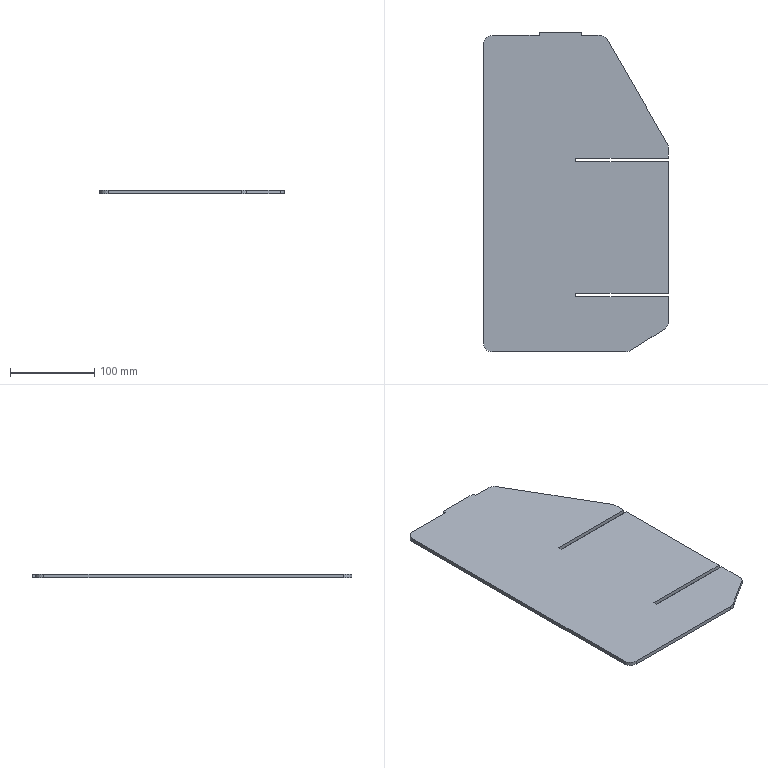Part | SolidWorks | features FlatPattern 1, SMBaseFlange 1, SheetMetal 1 | 1 solid | 26 faces | box 218.7 x 379.2 x 4.5 mm | volume 340357 mm3 | plane 20 | cylinder 6 | commonest cylinder face diameters 20 x6
STEP:
#1=CARTESIAN_POINT('',(18.5,-249.8,0.));
#2=VERTEX_POINT('',#1);
#3=CARTESIAN_POINT('',(8.5,-259.8,0.));
#4=VERTEX_POINT('',#3);
#5=CARTESIAN_POINT('',(18.5,-259.8,0.));
#6=DIRECTION('',(0.,0.,1.));
#7=DIRECTION('',(1.,0.,0.));
#8=AXIS2_PLACEMENT_3D('',#5,#6,#7);
#9=CIRCLE('',#8,10.);
#10=EDGE_CURVE('',#2,#4,#9,.T.);
#11=ORIENTED_EDGE('',*,*,#10,.F.);
#12=CARTESIAN_POINT('',(18.5,-249.8,-4.5));
#13=VERTEX_POINT('',#12);
#14=CARTESIAN_POINT('',(18.5,-249.8,-4.5));
#15=DIRECTION('',(0.,0.,1.));
#16=VECTOR('',#15,1000.);
#17=LINE('',#14,#16);
#18=EDGE_CURVE('',#13,#2,#17,.T.);
#19=ORIENTED_EDGE('',*,*,#18,.F.);
#20=CARTESIAN_POINT('',(8.5,-259.8,-4.5));
#21=VERTEX_POINT('',#20);
#22=CARTESIAN_POINT('',(18.5,-259.8,-4.5));
#23=DIRECTION('',(0.,0.,1.));
#24=DIRECTION('',(1.,0.,0.));
#25=AXIS2_PLACEMENT_3D('',#22,#23,#24);
#26=CIRCLE('',#25,10.);
#27=EDGE_CURVE('',#13,#21,#26,.T.);
#28=ORIENTED_EDGE('',*,*,#27,.T.);
#29=CARTESIAN_POINT('',(8.5,-259.8,-4.5));
#30=DIRECTION('',(0.,0.,1.));
#31=VECTOR('',#30,1000.);
#32=LINE('',#29,#31);
#33=EDGE_CURVE('',#21,#4,#32,.T.);
#34=ORIENTED_EDGE('',*,*,#33,.T.);
#35=EDGE_LOOP('',(#11,#19,#28,#34));
#36=FACE_OUTER_BOUND('',#35,.T.);
#37=CARTESIAN_POINT('',(18.5,-259.8,-4.5));
#38=DIRECTION('',(0.,0.,1.));
#39=DIRECTION('',(1.,0.,0.));
#40=AXIS2_PLACEMENT_3D('',#37,#38,#39);
#41=CYLINDRICAL_SURFACE('',#40,10.);
#42=ADVANCED_FACE('',(#36),#41,.T.);
#43=CARTESIAN_POINT('',(74.2,-249.8,0.));
#44=VERTEX_POINT('',#43);
#45=CARTESIAN_POINT('',(18.5,-249.8,0.));
#46=DIRECTION('',(-1.,0.,0.));
#47=VECTOR('',#46,1000.);
#48=LINE('',#45,#47);
#49=EDGE_CURVE('',#44,#2,#48,.T.);
#50=ORIENTED_EDGE('',*,*,#49,.F.);
#51=CARTESIAN_POINT('',(74.2,-249.8,-4.5));
#52=VERTEX_POINT('',#51);
#53=CARTESIAN_POINT('',(74.2,-249.8,-4.5));
#54=DIRECTION('',(0.,0.,1.));
#55=VECTOR('',#54,1000.);
#56=LINE('',#53,#55);
#57=EDGE_CURVE('',#52,#44,#56,.T.);
#58=ORIENTED_EDGE('',*,*,#57,.F.);
#59=CARTESIAN_POINT('',(18.5,-249.8,-4.5));
#60=DIRECTION('',(-1.,0.,0.));
#61=VECTOR('',#60,1000.);
#62=LINE('',#59,#61);
#63=EDGE_CURVE('',#52,#13,#62,.T.);
#64=ORIENTED_EDGE('',*,*,#63,.T.);
#65=ORIENTED_EDGE('',*,*,#18,.T.);
#66=EDGE_LOOP('',(#50,#58,#64,#65));
#67=FACE_OUTER_BOUND('',#66,.T.);
#68=CARTESIAN_POINT('',(18.5,-249.8,-4.5));
#69=DIRECTION('',(0.,1.,0.));
#70=DIRECTION('',(-1.,0.,0.));
#71=AXIS2_PLACEMENT_3D('',#68,#69,#70);
#72=PLANE('',#71);
#73=ADVANCED_FACE('',(#67),#72,.T.);
#74=CARTESIAN_POINT('',(74.2,-245.8,0.));
#75=VERTEX_POINT('',#74);
#76=CARTESIAN_POINT('',(74.2,-245.8,0.));
#77=DIRECTION('',(0.,-1.,0.));
#78=VECTOR('',#77,1000.);
#79=LINE('',#76,#78);
#80=EDGE_CURVE('',#75,#44,#79,.T.);
#81=ORIENTED_EDGE('',*,*,#80,.F.);
#82=CARTESIAN_POINT('',(74.2,-245.8,-4.5));
#83=VERTEX_POINT('',#82);
#84=CARTESIAN_POINT('',(74.2,-245.8,-4.5));
#85=DIRECTION('',(0.,0.,1.));
#86=VECTOR('',#85,1000.);
#87=LINE('',#84,#86);
#88=EDGE_CURVE('',#83,#75,#87,.T.);
#89=ORIENTED_EDGE('',*,*,#88,.F.);
#90=CARTESIAN_POINT('',(74.2,-245.8,-4.5));
#91=DIRECTION('',(0.,-1.,0.));
#92=VECTOR('',#91,1000.);
#93=LINE('',#90,#92);
#94=EDGE_CURVE('',#83,#52,#93,.T.);
#95=ORIENTED_EDGE('',*,*,#94,.T.);
#96=ORIENTED_EDGE('',*,*,#57,.T.);
#97=EDGE_LOOP('',(#81,#89,#95,#96));
#98=FACE_OUTER_BOUND('',#97,.T.);
#99=CARTESIAN_POINT('',(74.2,-245.8,-4.5));
#100=DIRECTION('',(-1.,0.,0.));
#101=DIRECTION('',(0.,0.,1.));
#102=AXIS2_PLACEMENT_3D('',#99,#100,#101);
#103=PLANE('',#102);
#104=ADVANCED_FACE('',(#98),#103,.T.);
#105=CARTESIAN_POINT('',(124.2,-245.8,0.));
#106=VERTEX_POINT('',#105);
#107=CARTESIAN_POINT('',(124.2,-245.8,0.));
#108=DIRECTION('',(-1.,0.,0.));
#109=VECTOR('',#108,1000.);
#110=LINE('',#107,#109);
#111=EDGE_CURVE('',#106,#75,#110,.T.);
#112=ORIENTED_EDGE('',*,*,#111,.F.);
#113=CARTESIAN_POINT('',(124.2,-245.8,-4.5));
#114=VERTEX_POINT('',#113);
#115=CARTESIAN_POINT('',(124.2,-245.8,-4.5));
#116=DIRECTION('',(0.,0.,1.));
#117=VECTOR('',#116,1000.);
#118=LINE('',#115,#117);
#119=EDGE_CURVE('',#114,#106,#118,.T.);
#120=ORIENTED_EDGE('',*,*,#119,.F.);
#121=CARTESIAN_POINT('',(124.2,-245.8,-4.5));
#122=DIRECTION('',(-1.,0.,0.));
#123=VECTOR('',#122,1000.);
#124=LINE('',#121,#123);
#125=EDGE_CURVE('',#114,#83,#124,.T.);
#126=ORIENTED_EDGE('',*,*,#125,.T.);
#127=ORIENTED_EDGE('',*,*,#88,.T.);
#128=EDGE_LOOP('',(#112,#120,#126,#127));
#129=FACE_OUTER_BOUND('',#128,.T.);
#130=CARTESIAN_POINT('',(124.2,-245.8,-4.5));
#131=DIRECTION('',(0.,1.,0.));
#132=DIRECTION('',(-1.,0.,0.));
#133=AXIS2_PLACEMENT_3D('',#130,#131,#132);
#134=PLANE('',#133);
#135=ADVANCED_FACE('',(#129),#134,.T.);
#136=CARTESIAN_POINT('',(124.2,-249.8,0.));
#137=VERTEX_POINT('',#136);
#138=CARTESIAN_POINT('',(124.2,-249.8,0.));
#139=DIRECTION('',(0.,1.,0.));
#140=VECTOR('',#139,1000.);
#141=LINE('',#138,#140);
#142=EDGE_CURVE('',#137,#106,#141,.T.);
#143=ORIENTED_EDGE('',*,*,#142,.F.);
#144=CARTESIAN_POINT('',(124.2,-249.8,-4.5));
#145=VERTEX_POINT('',#144);
#146=CARTESIAN_POINT('',(124.2,-249.8,-4.5));
#147=DIRECTION('',(0.,0.,1.));
#148=VECTOR('',#147,1000.);
#149=LINE('',#146,#148);
#150=EDGE_CURVE('',#145,#137,#149,.T.);
#151=ORIENTED_EDGE('',*,*,#150,.F.);
#152=CARTESIAN_POINT('',(124.2,-249.8,-4.5));
#153=DIRECTION('',(0.,1.,0.));
#154=VECTOR('',#153,1000.);
#155=LINE('',#152,#154);
#156=EDGE_CURVE('',#145,#114,#155,.T.);
#157=ORIENTED_EDGE('',*,*,#156,.T.);
#158=ORIENTED_EDGE('',*,*,#119,.T.);
#159=EDGE_LOOP('',(#143,#151,#157,#158));
#160=FACE_OUTER_BOUND('',#159,.T.);
#161=CARTESIAN_POINT('',(124.2,-249.8,-4.5));
#162=DIRECTION('',(1.,0.,0.));
#163=DIRECTION('',(0.,0.,-1.));
#164=AXIS2_PLACEMENT_3D('',#161,#162,#163);
#165=PLANE('',#164);
#166=ADVANCED_FACE('',(#160),#165,.T.);
#167=CARTESIAN_POINT('',(146.371,-249.8,0.));
#168=VERTEX_POINT('',#167);
#169=CARTESIAN_POINT('',(124.2,-249.8,0.));
#170=DIRECTION('',(-1.,0.,0.));
#171=VECTOR('',#170,1000.);
#172=LINE('',#169,#171);
#173=EDGE_CURVE('',#168,#137,#172,.T.);
#174=ORIENTED_EDGE('',*,*,#173,.F.);
#175=CARTESIAN_POINT('',(146.371,-249.8,-4.5));
#176=VERTEX_POINT('',#175);
#177=CARTESIAN_POINT('',(146.371,-249.8,-4.5));
#178=DIRECTION('',(0.,0.,1.));
#179=VECTOR('',#178,1000.);
#180=LINE('',#177,#179);
#181=EDGE_CURVE('',#176,#168,#180,.T.);
#182=ORIENTED_EDGE('',*,*,#181,.F.);
#183=CARTESIAN_POINT('',(124.2,-249.8,-4.5));
#184=DIRECTION('',(-1.,0.,0.));
#185=VECTOR('',#184,1000.);
#186=LINE('',#183,#185);
#187=EDGE_CURVE('',#176,#145,#186,.T.);
#188=ORIENTED_EDGE('',*,*,#187,.T.);
#189=ORIENTED_EDGE('',*,*,#150,.T.);
#190=EDGE_LOOP('',(#174,#182,#188,#189));
#191=FACE_OUTER_BOUND('',#190,.T.);
#192=CARTESIAN_POINT('',(124.2,-249.8,-4.5));
#193=DIRECTION('',(0.,1.,0.));
#194=DIRECTION('',(0.,0.,1.));
#195=AXIS2_PLACEMENT_3D('',#192,#193,#194);
#196=PLANE('',#195);
#197=ADVANCED_FACE('',(#191),#196,.T.);
#198=CARTESIAN_POINT('',(155.031,-254.8,0.));
#199=VERTEX_POINT('',#198);
#200=CARTESIAN_POINT('',(146.371,-259.8,0.));
#201=DIRECTION('',(0.,0.,1.));
#202=DIRECTION('',(-1.,0.,0.));
#203=AXIS2_PLACEMENT_3D('',#200,#201,#202);
#204=CIRCLE('',#203,10.);
#205=EDGE_CURVE('',#199,#168,#204,.T.);
#206=ORIENTED_EDGE('',*,*,#205,.F.);
#207=CARTESIAN_POINT('',(155.031,-254.8,-4.5));
#208=VERTEX_POINT('',#207);
#209=CARTESIAN_POINT('',(155.031,-254.8,-4.5));
#210=DIRECTION('',(0.,0.,1.));
#211=VECTOR('',#210,1000.);
#212=LINE('',#209,#211);
#213=EDGE_CURVE('',#208,#199,#212,.T.);
#214=ORIENTED_EDGE('',*,*,#213,.F.);
#215=CARTESIAN_POINT('',(146.371,-259.8,-4.5));
#216=DIRECTION('',(0.,0.,1.));
#217=DIRECTION('',(-1.,0.,0.));
#218=AXIS2_PLACEMENT_3D('',#215,#216,#217);
#219=CIRCLE('',#218,10.);
#220=EDGE_CURVE('',#208,#176,#219,.T.);
#221=ORIENTED_EDGE('',*,*,#220,.T.);
#222=ORIENTED_EDGE('',*,*,#181,.T.);
#223=EDGE_LOOP('',(#206,#214,#221,#222));
#224=FACE_OUTER_BOUND('',#223,.T.);
#225=CARTESIAN_POINT('',(146.371,-259.8,-4.5));
#226=DIRECTION('',(0.,0.,1.));
#227=DIRECTION('',(1.,0.,0.));
#228=AXIS2_PLACEMENT_3D('',#225,#226,#227);
#229=CYLINDRICAL_SURFACE('',#228,10.);
#230=ADVANCED_FACE('',(#224),#229,.T.);
#231=CARTESIAN_POINT('',(225.86,-377.479,0.));
#232=VERTEX_POINT('',#231);
#233=CARTESIAN_POINT('',(155.031,-254.8,0.));
#234=DIRECTION('',(-0.5,0.866,0.));
#235=VECTOR('',#234,1000.);
#236=LINE('',#233,#235);
#237=EDGE_CURVE('',#232,#199,#236,.T.);
#238=ORIENTED_EDGE('',*,*,#237,.F.);
#239=CARTESIAN_POINT('',(225.86,-377.479,-4.5));
#240=VERTEX_POINT('',#239);
#241=CARTESIAN_POINT('',(225.86,-377.479,-4.5));
#242=DIRECTION('',(0.,0.,1.));
#243=VECTOR('',#242,1000.);
#244=LINE('',#241,#243);
#245=EDGE_CURVE('',#240,#232,#244,.T.);
#246=ORIENTED_EDGE('',*,*,#245,.F.);
#247=CARTESIAN_POINT('',(155.031,-254.8,-4.5));
#248=DIRECTION('',(-0.5,0.866,0.));
#249=VECTOR('',#248,1000.);
#250=LINE('',#247,#249);
#251=EDGE_CURVE('',#240,#208,#250,.T.);
#252=ORIENTED_EDGE('',*,*,#251,.T.);
#253=ORIENTED_EDGE('',*,*,#213,.T.);
#254=EDGE_LOOP('',(#238,#246,#252,#253));
#255=FACE_OUTER_BOUND('',#254,.T.);
#256=CARTESIAN_POINT('',(155.031,-254.8,-4.5));
#257=DIRECTION('',(0.866,0.5,0.));
#258=DIRECTION('',(-0.5,0.866,0.));
#259=AXIS2_PLACEMENT_3D('',#256,#257,#258);
#260=PLANE('',#259);
#261=ADVANCED_FACE('',(#255),#260,.T.);
#262=CARTESIAN_POINT('',(227.2,-382.479,0.));
#263=VERTEX_POINT('',#262);
#264=CARTESIAN_POINT('',(217.2,-382.479,0.));
#265=DIRECTION('',(0.,0.,1.));
#266=DIRECTION('',(1.,0.,0.));
#267=AXIS2_PLACEMENT_3D('',#264,#265,#266);
#268=CIRCLE('',#267,10.);
#269=EDGE_CURVE('',#263,#232,#268,.T.);
#270=ORIENTED_EDGE('',*,*,#269,.F.);
#271=CARTESIAN_POINT('',(227.2,-382.479,-4.5));
#272=VERTEX_POINT('',#271);
#273=CARTESIAN_POINT('',(227.2,-382.479,-4.5));
#274=DIRECTION('',(0.,0.,1.));
#275=VECTOR('',#274,1000.);
#276=LINE('',#273,#275);
#277=EDGE_CURVE('',#272,#263,#276,.T.);
#278=ORIENTED_EDGE('',*,*,#277,.F.);
#279=CARTESIAN_POINT('',(217.2,-382.479,-4.5));
#280=DIRECTION('',(0.,0.,1.));
#281=DIRECTION('',(1.,0.,0.));
#282=AXIS2_PLACEMENT_3D('',#279,#280,#281);
#283=CIRCLE('',#282,10.);
#284=EDGE_CURVE('',#272,#240,#283,.T.);
#285=ORIENTED_EDGE('',*,*,#284,.T.);
#286=ORIENTED_EDGE('',*,*,#245,.T.);
#287=EDGE_LOOP('',(#270,#278,#285,#286));
#288=FACE_OUTER_BOUND('',#287,.T.);
#289=CARTESIAN_POINT('',(217.2,-382.479,-4.5));
#290=DIRECTION('',(0.,0.,1.));
#291=DIRECTION('',(1.,0.,0.));
#292=AXIS2_PLACEMENT_3D('',#289,#290,#291);
#293=CYLINDRICAL_SURFACE('',#292,10.);
#294=ADVANCED_FACE('',(#288),#293,.T.);
#295=CARTESIAN_POINT('',(227.2,-395.3,0.));
#296=VERTEX_POINT('',#295);
#297=CARTESIAN_POINT('',(227.2,-382.479,0.));
#298=DIRECTION('',(0.,1.,0.));
#299=VECTOR('',#298,1000.);
#300=LINE('',#297,#299);
#301=EDGE_CURVE('',#296,#263,#300,.T.);
#302=ORIENTED_EDGE('',*,*,#301,.F.);
#303=CARTESIAN_POINT('',(227.2,-395.3,-4.5));
#304=VERTEX_POINT('',#303);
#305=CARTESIAN_POINT('',(227.2,-395.3,-4.5));
#306=DIRECTION('',(0.,0.,1.));
#307=VECTOR('',#306,1000.);
#308=LINE('',#305,#307);
#309=EDGE_CURVE('',#304,#296,#308,.T.);
#310=ORIENTED_EDGE('',*,*,#309,.F.);
#311=CARTESIAN_POINT('',(227.2,-382.479,-4.5));
#312=DIRECTION('',(0.,1.,0.));
#313=VECTOR('',#312,1000.);
#314=LINE('',#311,#313);
#315=EDGE_CURVE('',#304,#272,#314,.T.);
#316=ORIENTED_EDGE('',*,*,#315,.T.);
#317=ORIENTED_EDGE('',*,*,#277,.T.);
#318=EDGE_LOOP('',(#302,#310,#316,#317));
#319=FACE_OUTER_BOUND('',#318,.T.);
#320=CARTESIAN_POINT('',(227.2,-382.479,-4.5));
#321=DIRECTION('',(1.,0.,0.));
#322=DIRECTION('',(0.,0.,-1.));
#323=AXIS2_PLACEMENT_3D('',#320,#321,#322);
#324=PLANE('',#323);
#325=ADVANCED_FACE('',(#319),#324,.T.);
#326=CARTESIAN_POINT('',(117.7,-395.3,0.));
#327=VERTEX_POINT('',#326);
#328=CARTESIAN_POINT('',(227.2,-395.3,0.));
#329=DIRECTION('',(1.,0.,0.));
#330=VECTOR('',#329,1000.);
#331=LINE('',#328,#330);
#332=EDGE_CURVE('',#327,#296,#331,.T.);
#333=ORIENTED_EDGE('',*,*,#332,.F.);
#334=CARTESIAN_POINT('',(117.7,-395.3,-4.5));
#335=VERTEX_POINT('',#334);
#336=CARTESIAN_POINT('',(117.7,-395.3,-4.5));
#337=DIRECTION('',(0.,0.,1.));
#338=VECTOR('',#337,1000.);
#339=LINE('',#336,#338);
#340=EDGE_CURVE('',#335,#327,#339,.T.);
#341=ORIENTED_EDGE('',*,*,#340,.F.);
#342=CARTESIAN_POINT('',(227.2,-395.3,-4.5));
#343=DIRECTION('',(1.,0.,0.));
#344=VECTOR('',#343,1000.);
#345=LINE('',#342,#344);
#346=EDGE_CURVE('',#335,#304,#345,.T.);
#347=ORIENTED_EDGE('',*,*,#346,.T.);
#348=ORIENTED_EDGE('',*,*,#309,.T.);
#349=EDGE_LOOP('',(#333,#341,#347,#348));
#350=FACE_OUTER_BOUND('',#349,.T.);
#351=CARTESIAN_POINT('',(227.2,-395.3,-4.5));
#352=DIRECTION('',(0.,-1.,0.));
#353=DIRECTION('',(1.,0.,0.));
#354=AXIS2_PLACEMENT_3D('',#351,#352,#353);
#355=PLANE('',#354);
#356=ADVANCED_FACE('',(#350),#355,.T.);
#357=CARTESIAN_POINT('',(117.7,-399.8,0.));
#358=VERTEX_POINT('',#357);
#359=CARTESIAN_POINT('',(117.7,-395.3,0.));
#360=DIRECTION('',(0.,1.,0.));
#361=VECTOR('',#360,1000.);
#362=LINE('',#359,#361);
#363=EDGE_CURVE('',#358,#327,#362,.T.);
#364=ORIENTED_EDGE('',*,*,#363,.F.);
#365=CARTESIAN_POINT('',(117.7,-399.8,-4.5));
#366=VERTEX_POINT('',#365);
#367=CARTESIAN_POINT('',(117.7,-399.8,-4.5));
#368=DIRECTION('',(0.,0.,1.));
#369=VECTOR('',#368,1000.);
#370=LINE('',#367,#369);
#371=EDGE_CURVE('',#366,#358,#370,.T.);
#372=ORIENTED_EDGE('',*,*,#371,.F.);
#373=CARTESIAN_POINT('',(117.7,-395.3,-4.5));
#374=DIRECTION('',(0.,1.,0.));
#375=VECTOR('',#374,1000.);
#376=LINE('',#373,#375);
#377=EDGE_CURVE('',#366,#335,#376,.T.);
#378=ORIENTED_EDGE('',*,*,#377,.T.);
#379=ORIENTED_EDGE('',*,*,#340,.T.);
#380=EDGE_LOOP('',(#364,#372,#378,#379));
#381=FACE_OUTER_BOUND('',#380,.T.);
#382=CARTESIAN_POINT('',(117.7,-395.3,-4.5));
#383=DIRECTION('',(1.,0.,0.));
#384=DIRECTION('',(0.,0.,-1.));
#385=AXIS2_PLACEMENT_3D('',#382,#383,#384);
#386=PLANE('',#385);
#387=ADVANCED_FACE('',(#381),#386,.T.);
#388=CARTESIAN_POINT('',(227.2,-399.8,0.));
#389=VERTEX_POINT('',#388);
#390=CARTESIAN_POINT('',(117.7,-399.8,0.));
#391=DIRECTION('',(-1.,0.,0.));
#392=VECTOR('',#391,1000.);
#393=LINE('',#390,#392);
#394=EDGE_CURVE('',#389,#358,#393,.T.);
#395=ORIENTED_EDGE('',*,*,#394,.F.);
#396=CARTESIAN_POINT('',(227.2,-399.8,-4.5));
#397=VERTEX_POINT('',#396);
#398=CARTESIAN_POINT('',(227.2,-399.8,-4.5));
#399=DIRECTION('',(0.,0.,1.));
#400=VECTOR('',#399,1000.);
#401=LINE('',#398,#400);
#402=EDGE_CURVE('',#397,#389,#401,.T.);
#403=ORIENTED_EDGE('',*,*,#402,.F.);
#404=CARTESIAN_POINT('',(117.7,-399.8,-4.5));
#405=DIRECTION('',(-1.,0.,0.));
#406=VECTOR('',#405,1000.);
#407=LINE('',#404,#406);
#408=EDGE_CURVE('',#397,#366,#407,.T.);
#409=ORIENTED_EDGE('',*,*,#408,.T.);
#410=ORIENTED_EDGE('',*,*,#371,.T.);
#411=EDGE_LOOP('',(#395,#403,#409,#410));
#412=FACE_OUTER_BOUND('',#411,.T.);
#413=CARTESIAN_POINT('',(117.7,-399.8,-4.5));
#414=DIRECTION('',(0.,1.,0.));
#415=DIRECTION('',(-1.,0.,0.));
#416=AXIS2_PLACEMENT_3D('',#413,#414,#415);
#417=PLANE('',#416);
#418=ADVANCED_FACE('',(#412),#417,.T.);
#419=CARTESIAN_POINT('',(227.2,-555.3,0.));
#420=VERTEX_POINT('',#419);
#421=CARTESIAN_POINT('',(227.2,-399.8,0.));
#422=DIRECTION('',(0.,1.,0.));
#423=VECTOR('',#422,1000.);
#424=LINE('',#421,#423);
#425=EDGE_CURVE('',#420,#389,#424,.T.);
#426=ORIENTED_EDGE('',*,*,#425,.F.);
#427=CARTESIAN_POINT('',(227.2,-555.3,-4.5));
#428=VERTEX_POINT('',#427);
#429=CARTESIAN_POINT('',(227.2,-555.3,-4.5));
#430=DIRECTION('',(0.,0.,1.));
#431=VECTOR('',#430,1000.);
#432=LINE('',#429,#431);
#433=EDGE_CURVE('',#428,#420,#432,.T.);
#434=ORIENTED_EDGE('',*,*,#433,.F.);
#435=CARTESIAN_POINT('',(227.2,-399.8,-4.5));
#436=DIRECTION('',(0.,1.,0.));
#437=VECTOR('',#436,1000.);
#438=LINE('',#435,#437);
#439=EDGE_CURVE('',#428,#397,#438,.T.);
#440=ORIENTED_EDGE('',*,*,#439,.T.);
#441=ORIENTED_EDGE('',*,*,#402,.T.);
#442=EDGE_LOOP('',(#426,#434,#440,#441));
#443=FACE_OUTER_BOUND('',#442,.T.);
#444=CARTESIAN_POINT('',(227.2,-399.8,-4.5));
#445=DIRECTION('',(1.,0.,0.));
#446=DIRECTION('',(0.,1.,0.));
#447=AXIS2_PLACEMENT_3D('',#444,#445,#446);
#448=PLANE('',#447);
#449=ADVANCED_FACE('',(#443),#448,.T.);
#450=CARTESIAN_POINT('',(117.7,-555.3,0.));
#451=VERTEX_POINT('',#450);
#452=CARTESIAN_POINT('',(227.2,-555.3,0.));
#453=DIRECTION('',(1.,0.,0.));
#454=VECTOR('',#453,1000.);
#455=LINE('',#452,#454);
#456=EDGE_CURVE('',#451,#420,#455,.T.);
#457=ORIENTED_EDGE('',*,*,#456,.F.);
#458=CARTESIAN_POINT('',(117.7,-555.3,-4.5));
#459=VERTEX_POINT('',#458);
#460=CARTESIAN_POINT('',(117.7,-555.3,-4.5));
#461=DIRECTION('',(0.,0.,1.));
#462=VECTOR('',#461,1000.);
#463=LINE('',#460,#462);
#464=EDGE_CURVE('',#459,#451,#463,.T.);
#465=ORIENTED_EDGE('',*,*,#464,.F.);
#466=CARTESIAN_POINT('',(227.2,-555.3,-4.5));
#467=DIRECTION('',(1.,0.,0.));
#468=VECTOR('',#467,1000.);
#469=LINE('',#466,#468);
#470=EDGE_CURVE('',#459,#428,#469,.T.);
#471=ORIENTED_EDGE('',*,*,#470,.T.);
#472=ORIENTED_EDGE('',*,*,#433,.T.);
#473=EDGE_LOOP('',(#457,#465,#471,#472));
#474=FACE_OUTER_BOUND('',#473,.T.);
#475=CARTESIAN_POINT('',(227.2,-555.3,-4.5));
#476=DIRECTION('',(0.,-1.,0.));
#477=DIRECTION('',(0.,0.,-1.));
#478=AXIS2_PLACEMENT_3D('',#475,#476,#477);
#479=PLANE('',#478);
#480=ADVANCED_FACE('',(#474),#479,.T.);
#481=CARTESIAN_POINT('',(117.7,-559.8,0.));
#482=VERTEX_POINT('',#481);
#483=CARTESIAN_POINT('',(117.7,-555.3,0.));
#484=DIRECTION('',(0.,1.,0.));
#485=VECTOR('',#484,1000.);
#486=LINE('',#483,#485);
#487=EDGE_CURVE('',#482,#451,#486,.T.);
#488=ORIENTED_EDGE('',*,*,#487,.F.);
#489=CARTESIAN_POINT('',(117.7,-559.8,-4.5));
#490=VERTEX_POINT('',#489);
#491=CARTESIAN_POINT('',(117.7,-559.8,-4.5));
#492=DIRECTION('',(0.,0.,1.));
#493=VECTOR('',#492,1000.);
#494=LINE('',#491,#493);
#495=EDGE_CURVE('',#490,#482,#494,.T.);
#496=ORIENTED_EDGE('',*,*,#495,.F.);
#497=CARTESIAN_POINT('',(117.7,-555.3,-4.5));
#498=DIRECTION('',(0.,1.,0.));
#499=VECTOR('',#498,1000.);
#500=LINE('',#497,#499);
#501=EDGE_CURVE('',#490,#459,#500,.T.);
#502=ORIENTED_EDGE('',*,*,#501,.T.);
#503=ORIENTED_EDGE('',*,*,#464,.T.);
#504=EDGE_LOOP('',(#488,#496,#502,#503));
#505=FACE_OUTER_BOUND('',#504,.T.);
#506=CARTESIAN_POINT('',(117.7,-555.3,-4.5));
#507=DIRECTION('',(1.,0.,0.));
#508=DIRECTION('',(0.,1.,0.));
#509=AXIS2_PLACEMENT_3D('',#506,#507,#508);
#510=PLANE('',#509);
#511=ADVANCED_FACE('',(#505),#510,.T.);
#512=CARTESIAN_POINT('',(227.2,-559.8,0.));
#513=VERTEX_POINT('',#512);
#514=CARTESIAN_POINT('',(117.7,-559.8,0.));
#515=DIRECTION('',(-1.,0.,0.));
#516=VECTOR('',#515,1000.);
#517=LINE('',#514,#516);
#518=EDGE_CURVE('',#513,#482,#517,.T.);
#519=ORIENTED_EDGE('',*,*,#518,.F.);
#520=CARTESIAN_POINT('',(227.2,-559.8,-4.5));
#521=VERTEX_POINT('',#520);
#522=CARTESIAN_POINT('',(227.2,-559.8,-4.5));
#523=DIRECTION('',(0.,0.,1.));
#524=VECTOR('',#523,1000.);
#525=LINE('',#522,#524);
#526=EDGE_CURVE('',#521,#513,#525,.T.);
#527=ORIENTED_EDGE('',*,*,#526,.F.);
#528=CARTESIAN_POINT('',(117.7,-559.8,-4.5));
#529=DIRECTION('',(-1.,0.,0.));
#530=VECTOR('',#529,1000.);
#531=LINE('',#528,#530);
#532=EDGE_CURVE('',#521,#490,#531,.T.);
#533=ORIENTED_EDGE('',*,*,#532,.T.);
#534=ORIENTED_EDGE('',*,*,#495,.T.);
#535=EDGE_LOOP('',(#519,#527,#533,#534));
#536=FACE_OUTER_BOUND('',#535,.T.);
#537=CARTESIAN_POINT('',(117.7,-559.8,-4.5));
#538=DIRECTION('',(0.,1.,0.));
#539=DIRECTION('',(0.,0.,1.));
#540=AXIS2_PLACEMENT_3D('',#537,#538,#539);
#541=PLANE('',#540);
#542=ADVANCED_FACE('',(#536),#541,.T.);
#543=CARTESIAN_POINT('',(227.2,-589.69,0.));
#544=VERTEX_POINT('',#543);
#545=CARTESIAN_POINT('',(227.2,-559.8,0.));
#546=DIRECTION('',(0.,1.,0.));
#547=VECTOR('',#546,1000.);
#548=LINE('',#545,#547);
#549=EDGE_CURVE('',#544,#513,#548,.T.);
#550=ORIENTED_EDGE('',*,*,#549,.F.);
#551=CARTESIAN_POINT('',(227.2,-589.69,-4.5));
#552=VERTEX_POINT('',#551);
#553=CARTESIAN_POINT('',(227.2,-589.69,-4.5));
#554=DIRECTION('',(0.,0.,1.));
#555=VECTOR('',#554,1000.);
#556=LINE('',#553,#555);
#557=EDGE_CURVE('',#552,#544,#556,.T.);
#558=ORIENTED_EDGE('',*,*,#557,.F.);
#559=CARTESIAN_POINT('',(227.2,-559.8,-4.5));
#560=DIRECTION('',(0.,1.,0.));
#561=VECTOR('',#560,1000.);
#562=LINE('',#559,#561);
#563=EDGE_CURVE('',#552,#521,#562,.T.);
#564=ORIENTED_EDGE('',*,*,#563,.T.);
#565=ORIENTED_EDGE('',*,*,#526,.T.);
#566=EDGE_LOOP('',(#550,#558,#564,#565));
#567=FACE_OUTER_BOUND('',#566,.T.);
#568=CARTESIAN_POINT('',(227.2,-559.8,-4.5));
#569=DIRECTION('',(1.,0.,0.));
#570=DIRECTION('',(0.,0.,-1.));
#571=AXIS2_PLACEMENT_3D('',#568,#569,#570);
#572=PLANE('',#571);
#573=ADVANCED_FACE('',(#567),#572,.T.);
#574=CARTESIAN_POINT('',(222.541,-598.143,0.));
#575=VERTEX_POINT('',#574);
#576=CARTESIAN_POINT('',(217.2,-589.69,0.));
#577=DIRECTION('',(0.,0.,1.));
#578=DIRECTION('',(-1.,0.,0.));
#579=AXIS2_PLACEMENT_3D('',#576,#577,#578);
#580=CIRCLE('',#579,10.);
#581=EDGE_CURVE('',#575,#544,#580,.T.);
#582=ORIENTED_EDGE('',*,*,#581,.F.);
#583=CARTESIAN_POINT('',(222.541,-598.143,-4.5));
#584=VERTEX_POINT('',#583);
#585=CARTESIAN_POINT('',(222.541,-598.143,-4.5));
#586=DIRECTION('',(0.,0.,1.));
#587=VECTOR('',#586,1000.);
#588=LINE('',#585,#587);
#589=EDGE_CURVE('',#584,#575,#588,.T.);
#590=ORIENTED_EDGE('',*,*,#589,.F.);
#591=CARTESIAN_POINT('',(217.2,-589.69,-4.5));
#592=DIRECTION('',(0.,0.,1.));
#593=DIRECTION('',(-1.,0.,0.));
#594=AXIS2_PLACEMENT_3D('',#591,#592,#593);
#595=CIRCLE('',#594,10.);
#596=EDGE_CURVE('',#584,#552,#595,.T.);
#597=ORIENTED_EDGE('',*,*,#596,.T.);
#598=ORIENTED_EDGE('',*,*,#557,.T.);
#599=EDGE_LOOP('',(#582,#590,#597,#598));
#600=FACE_OUTER_BOUND('',#599,.T.);
#601=CARTESIAN_POINT('',(217.2,-589.69,-4.5));
#602=DIRECTION('',(0.,0.,1.));
#603=DIRECTION('',(1.,0.,0.));
#604=AXIS2_PLACEMENT_3D('',#601,#602,#603);
#605=CYLINDRICAL_SURFACE('',#604,10.);
#606=ADVANCED_FACE('',(#600),#605,.T.);
#607=CARTESIAN_POINT('',(182.483,-623.454,0.));
#608=VERTEX_POINT('',#607);
#609=CARTESIAN_POINT('',(182.483,-623.454,0.));
#610=DIRECTION('',(0.8454,0.5342,0.));
#611=VECTOR('',#610,1000.);
#612=LINE('',#609,#611);
#613=EDGE_CURVE('',#608,#575,#612,.T.);
#614=ORIENTED_EDGE('',*,*,#613,.F.);
#615=CARTESIAN_POINT('',(182.483,-623.454,-4.5));
#616=VERTEX_POINT('',#615);
#617=CARTESIAN_POINT('',(182.483,-623.454,-4.5));
#618=DIRECTION('',(0.,0.,1.));
#619=VECTOR('',#618,1000.);
#620=LINE('',#617,#619);
#621=EDGE_CURVE('',#616,#608,#620,.T.);
#622=ORIENTED_EDGE('',*,*,#621,.F.);
#623=CARTESIAN_POINT('',(182.483,-623.454,-4.5));
#624=DIRECTION('',(0.8454,0.5342,0.));
#625=VECTOR('',#624,1000.);
#626=LINE('',#623,#625);
#627=EDGE_CURVE('',#616,#584,#626,.T.);
#628=ORIENTED_EDGE('',*,*,#627,.T.);
#629=ORIENTED_EDGE('',*,*,#589,.T.);
#630=EDGE_LOOP('',(#614,#622,#628,#629));
#631=FACE_OUTER_BOUND('',#630,.T.);
#632=CARTESIAN_POINT('',(182.483,-623.454,-4.5));
#633=DIRECTION('',(0.5342,-0.8454,0.));
#634=DIRECTION('',(0.8454,0.5342,0.));
#635=AXIS2_PLACEMENT_3D('',#632,#633,#634);
#636=PLANE('',#635);
#637=ADVANCED_FACE('',(#631),#636,.T.);
#638=CARTESIAN_POINT('',(177.142,-625.,0.));
#639=VERTEX_POINT('',#638);
#640=CARTESIAN_POINT('',(177.142,-615.,0.));
#641=DIRECTION('',(0.,0.,1.));
#642=DIRECTION('',(1.,0.,0.));
#643=AXIS2_PLACEMENT_3D('',#640,#641,#642);
#644=CIRCLE('',#643,10.);
#645=EDGE_CURVE('',#639,#608,#644,.T.);
#646=ORIENTED_EDGE('',*,*,#645,.F.);
#647=CARTESIAN_POINT('',(177.142,-625.,-4.5));
#648=VERTEX_POINT('',#647);
#649=CARTESIAN_POINT('',(177.142,-625.,-4.5));
#650=DIRECTION('',(0.,0.,1.));
#651=VECTOR('',#650,1000.);
#652=LINE('',#649,#651);
#653=EDGE_CURVE('',#648,#639,#652,.T.);
#654=ORIENTED_EDGE('',*,*,#653,.F.);
#655=CARTESIAN_POINT('',(177.142,-615.,-4.5));
#656=DIRECTION('',(0.,0.,1.));
#657=DIRECTION('',(1.,0.,0.));
#658=AXIS2_PLACEMENT_3D('',#655,#656,#657);
#659=CIRCLE('',#658,10.);
#660=EDGE_CURVE('',#648,#616,#659,.T.);
#661=ORIENTED_EDGE('',*,*,#660,.T.);
#662=ORIENTED_EDGE('',*,*,#621,.T.);
#663=EDGE_LOOP('',(#646,#654,#661,#662));
#664=FACE_OUTER_BOUND('',#663,.T.);
#665=CARTESIAN_POINT('',(177.142,-615.,-4.5));
#666=DIRECTION('',(0.,0.,1.));
#667=DIRECTION('',(1.,0.,0.));
#668=AXIS2_PLACEMENT_3D('',#665,#666,#667);
#669=CYLINDRICAL_SURFACE('',#668,10.);
#670=ADVANCED_FACE('',(#664),#669,.T.);
#671=CARTESIAN_POINT('',(18.5,-625.,0.));
#672=VERTEX_POINT('',#671);
#673=CARTESIAN_POINT('',(177.142,-625.,0.));
#674=DIRECTION('',(1.,0.,0.));
#675=VECTOR('',#674,1000.);
#676=LINE('',#673,#675);
#677=EDGE_CURVE('',#672,#639,#676,.T.);
#678=ORIENTED_EDGE('',*,*,#677,.F.);
#679=CARTESIAN_POINT('',(18.5,-625.,-4.5));
#680=VERTEX_POINT('',#679);
#681=CARTESIAN_POINT('',(18.5,-625.,-4.5));
#682=DIRECTION('',(0.,0.,1.));
#683=VECTOR('',#682,1000.);
#684=LINE('',#681,#683);
#685=EDGE_CURVE('',#680,#672,#684,.T.);
#686=ORIENTED_EDGE('',*,*,#685,.F.);
#687=CARTESIAN_POINT('',(177.142,-625.,-4.5));
#688=DIRECTION('',(1.,0.,0.));
#689=VECTOR('',#688,1000.);
#690=LINE('',#687,#689);
#691=EDGE_CURVE('',#680,#648,#690,.T.);
#692=ORIENTED_EDGE('',*,*,#691,.T.);
#693=ORIENTED_EDGE('',*,*,#653,.T.);
#694=EDGE_LOOP('',(#678,#686,#692,#693));
#695=FACE_OUTER_BOUND('',#694,.T.);
#696=CARTESIAN_POINT('',(177.142,-625.,-4.5));
#697=DIRECTION('',(0.,-1.,0.));
#698=DIRECTION('',(1.,0.,0.));
#699=AXIS2_PLACEMENT_3D('',#696,#697,#698);
#700=PLANE('',#699);
#701=ADVANCED_FACE('',(#695),#700,.T.);
#702=CARTESIAN_POINT('',(8.5,-615.,0.));
#703=VERTEX_POINT('',#702);
#704=CARTESIAN_POINT('',(18.5,-615.,0.));
#705=DIRECTION('',(0.,0.,1.));
#706=DIRECTION('',(1.,0.,0.));
#707=AXIS2_PLACEMENT_3D('',#704,#705,#706);
#708=CIRCLE('',#707,10.);
#709=EDGE_CURVE('',#703,#672,#708,.T.);
#710=ORIENTED_EDGE('',*,*,#709,.F.);
#711=CARTESIAN_POINT('',(8.5,-615.,-4.5));
#712=VERTEX_POINT('',#711);
#713=CARTESIAN_POINT('',(8.5,-615.,-4.5));
#714=DIRECTION('',(0.,0.,1.));
#715=VECTOR('',#714,1000.);
#716=LINE('',#713,#715);
#717=EDGE_CURVE('',#712,#703,#716,.T.);
#718=ORIENTED_EDGE('',*,*,#717,.F.);
#719=CARTESIAN_POINT('',(18.5,-615.,-4.5));
#720=DIRECTION('',(0.,0.,1.));
#721=DIRECTION('',(1.,0.,0.));
#722=AXIS2_PLACEMENT_3D('',#719,#720,#721);
#723=CIRCLE('',#722,10.);
#724=EDGE_CURVE('',#712,#680,#723,.T.);
#725=ORIENTED_EDGE('',*,*,#724,.T.);
#726=ORIENTED_EDGE('',*,*,#685,.T.);
#727=EDGE_LOOP('',(#710,#718,#725,#726));
#728=FACE_OUTER_BOUND('',#727,.T.);
#729=CARTESIAN_POINT('',(18.5,-615.,-4.5));
#730=DIRECTION('',(0.,0.,1.));
#731=DIRECTION('',(1.,0.,0.));
#732=AXIS2_PLACEMENT_3D('',#729,#730,#731);
#733=CYLINDRICAL_SURFACE('',#732,10.);
#734=ADVANCED_FACE('',(#728),#733,.T.);
#735=CARTESIAN_POINT('',(8.5,-615.,0.));
#736=DIRECTION('',(0.,-1.,0.));
#737=VECTOR('',#736,1000.);
#738=LINE('',#735,#737);
#739=EDGE_CURVE('',#4,#703,#738,.T.);
#740=ORIENTED_EDGE('',*,*,#739,.F.);
#741=ORIENTED_EDGE('',*,*,#33,.F.);
#742=CARTESIAN_POINT('',(8.5,-615.,-4.5));
#743=DIRECTION('',(0.,-1.,0.));
#744=VECTOR('',#743,1000.);
#745=LINE('',#742,#744);
#746=EDGE_CURVE('',#21,#712,#745,.T.);
#747=ORIENTED_EDGE('',*,*,#746,.T.);
#748=ORIENTED_EDGE('',*,*,#717,.T.);
#749=EDGE_LOOP('',(#740,#741,#747,#748));
#750=FACE_OUTER_BOUND('',#749,.T.);
#751=CARTESIAN_POINT('',(8.5,-615.,-4.5));
#752=DIRECTION('',(-1.,0.,0.));
#753=DIRECTION('',(0.,-1.,0.));
#754=AXIS2_PLACEMENT_3D('',#751,#752,#753);
#755=PLANE('',#754);
#756=ADVANCED_FACE('',(#750),#755,.T.);
#757=ORIENTED_EDGE('',*,*,#27,.F.);
#758=ORIENTED_EDGE('',*,*,#63,.F.);
#759=ORIENTED_EDGE('',*,*,#94,.F.);
#760=ORIENTED_EDGE('',*,*,#125,.F.);
#761=ORIENTED_EDGE('',*,*,#156,.F.);
#762=ORIENTED_EDGE('',*,*,#187,.F.);
#763=ORIENTED_EDGE('',*,*,#220,.F.);
#764=ORIENTED_EDGE('',*,*,#251,.F.);
#765=ORIENTED_EDGE('',*,*,#284,.F.);
#766=ORIENTED_EDGE('',*,*,#315,.F.);
#767=ORIENTED_EDGE('',*,*,#346,.F.);
#768=ORIENTED_EDGE('',*,*,#377,.F.);
#769=ORIENTED_EDGE('',*,*,#408,.F.);
#770=ORIENTED_EDGE('',*,*,#439,.F.);
#771=ORIENTED_EDGE('',*,*,#470,.F.);
#772=ORIENTED_EDGE('',*,*,#501,.F.);
#773=ORIENTED_EDGE('',*,*,#532,.F.);
#774=ORIENTED_EDGE('',*,*,#563,.F.);
#775=ORIENTED_EDGE('',*,*,#596,.F.);
#776=ORIENTED_EDGE('',*,*,#627,.F.);
#777=ORIENTED_EDGE('',*,*,#660,.F.);
#778=ORIENTED_EDGE('',*,*,#691,.F.);
#779=ORIENTED_EDGE('',*,*,#724,.F.);
#780=ORIENTED_EDGE('',*,*,#746,.F.);
#781=EDGE_LOOP('',(#757,#758,#759,#760,#761,#762,#763,#764,#765,#766,#767,#768,#769,#770,#771,#772,#773,#774,#775,#776,#777,#778,#779,#780));
#782=FACE_OUTER_BOUND('',#781,.T.);
#783=CARTESIAN_POINT('',(18.5,-259.8,-4.5));
#784=DIRECTION('',(0.,0.,1.));
#785=DIRECTION('',(1.,0.,0.));
#786=AXIS2_PLACEMENT_3D('',#783,#784,#785);
#787=PLANE('',#786);
#788=ADVANCED_FACE('',(#782),#787,.F.);
#789=ORIENTED_EDGE('',*,*,#10,.T.);
#790=ORIENTED_EDGE('',*,*,#739,.T.);
#791=ORIENTED_EDGE('',*,*,#709,.T.);
#792=ORIENTED_EDGE('',*,*,#677,.T.);
#793=ORIENTED_EDGE('',*,*,#645,.T.);
#794=ORIENTED_EDGE('',*,*,#613,.T.);
#795=ORIENTED_EDGE('',*,*,#581,.T.);
#796=ORIENTED_EDGE('',*,*,#549,.T.);
#797=ORIENTED_EDGE('',*,*,#518,.T.);
#798=ORIENTED_EDGE('',*,*,#487,.T.);
#799=ORIENTED_EDGE('',*,*,#456,.T.);
#800=ORIENTED_EDGE('',*,*,#425,.T.);
#801=ORIENTED_EDGE('',*,*,#394,.T.);
#802=ORIENTED_EDGE('',*,*,#363,.T.);
#803=ORIENTED_EDGE('',*,*,#332,.T.);
#804=ORIENTED_EDGE('',*,*,#301,.T.);
#805=ORIENTED_EDGE('',*,*,#269,.T.);
#806=ORIENTED_EDGE('',*,*,#237,.T.);
#807=ORIENTED_EDGE('',*,*,#205,.T.);
#808=ORIENTED_EDGE('',*,*,#173,.T.);
#809=ORIENTED_EDGE('',*,*,#142,.T.);
#810=ORIENTED_EDGE('',*,*,#111,.T.);
#811=ORIENTED_EDGE('',*,*,#80,.T.);
#812=ORIENTED_EDGE('',*,*,#49,.T.);
#813=EDGE_LOOP('',(#789,#790,#791,#792,#793,#794,#795,#796,#797,#798,#799,#800,#801,#802,#803,#804,#805,#806,#807,#808,#809,#810,#811,#812));
#814=FACE_OUTER_BOUND('',#813,.T.);
#815=CARTESIAN_POINT('',(18.5,-259.8,0.));
#816=DIRECTION('',(0.,0.,1.));
#817=DIRECTION('',(1.,0.,0.));
#818=AXIS2_PLACEMENT_3D('',#815,#816,#817);
#819=PLANE('',#818);
#820=ADVANCED_FACE('',(#814),#819,.T.);
#821=CLOSED_SHELL('',(#42,#73,#104,#135,#166,#197,#230,#261,#294,#325,#356,#387,#418,#449,#480,#511,#542,#573,#606,#637,#670,#701,#734,#756,#788,#820));
#822=MANIFOLD_SOLID_BREP('',#821);
#823=CARTESIAN_POINT('',(0.,0.,0.));
#824=DIRECTION('',(0.,0.,1.));
#825=DIRECTION('',(1.,0.,0.));
#826=AXIS2_PLACEMENT_3D('',#823,#824,#825);
#827=(LENGTH_UNIT()NAMED_UNIT(*)SI_UNIT(.MILLI.,.METRE.));
#828=UNCERTAINTY_MEASURE_WITH_UNIT(LENGTH_MEASURE(0.00001),#827,'','');
#829=(NAMED_UNIT(*)PLANE_ANGLE_UNIT()SI_UNIT($,.RADIAN.));
#830=(NAMED_UNIT(*)SI_UNIT($,.STERADIAN.)SOLID_ANGLE_UNIT());
#831=(GEOMETRIC_REPRESENTATION_CONTEXT(3)GLOBAL_UNCERTAINTY_ASSIGNED_CONTEXT((#828))GLOBAL_UNIT_ASSIGNED_CONTEXT((#827,#829,#830))REPRESENTATION_CONTEXT('',''));
#832=ADVANCED_BREP_SHAPE_REPRESENTATION('',(#822,#826),#831);